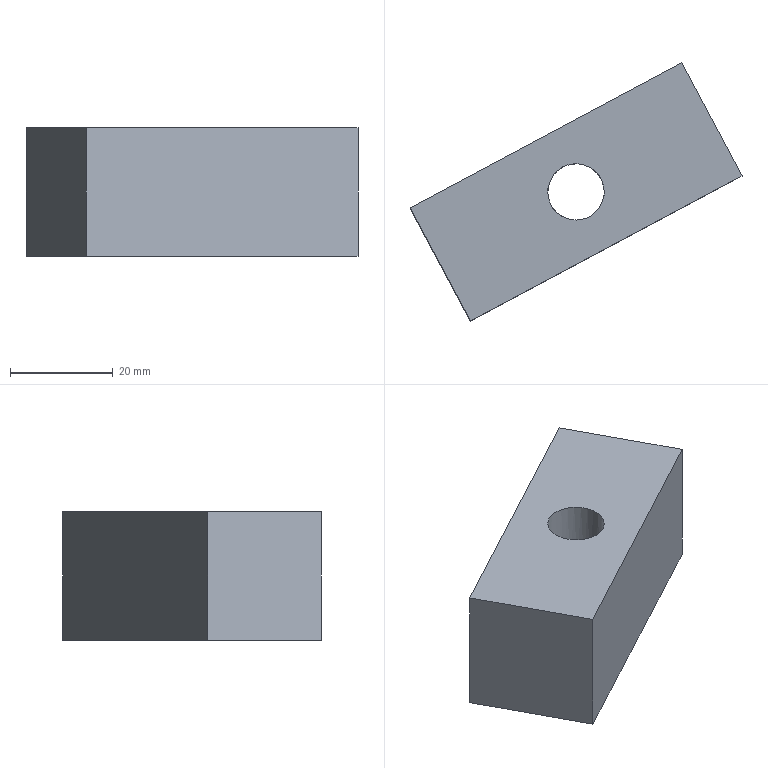Part | NX | features solid 2 | 1 solid | 9 faces | box 64.704 x 50.307 x 25 mm | volume 33211 mm3 | plane 7 | cylinder 2 | commonest cylinder face diameters 11 x1 18 x1
STEP:
#1=CARTESIAN_POINT('',(-802.083,-620.009,-2.));
#2=VERTEX_POINT('',#1);
#3=CARTESIAN_POINT('',(-749.151,-591.757,-2.));
#4=VERTEX_POINT('',#3);
#5=CARTESIAN_POINT('',(-802.083,-620.009,-2.));
#6=DIRECTION('',(0.8822,0.4709,0.));
#7=VECTOR('',#6,1000.);
#8=LINE('',#5,#7);
#9=EDGE_CURVE('',#2,#4,#8,.T.);
#10=ORIENTED_EDGE('',*,*,#9,.F.);
#11=CARTESIAN_POINT('',(-813.855,-597.954,-2.));
#12=VERTEX_POINT('',#11);
#13=CARTESIAN_POINT('',(-813.855,-597.954,-2.));
#14=DIRECTION('',(0.4709,-0.8822,0.));
#15=VECTOR('',#14,1000.);
#16=LINE('',#13,#15);
#17=EDGE_CURVE('',#12,#2,#16,.T.);
#18=ORIENTED_EDGE('',*,*,#17,.F.);
#19=CARTESIAN_POINT('',(-760.922,-569.702,-2.));
#20=VERTEX_POINT('',#19);
#21=CARTESIAN_POINT('',(-760.922,-569.702,-2.));
#22=DIRECTION('',(-0.8822,-0.4709,0.));
#23=VECTOR('',#22,1000.);
#24=LINE('',#21,#23);
#25=EDGE_CURVE('',#20,#12,#24,.T.);
#26=ORIENTED_EDGE('',*,*,#25,.F.);
#27=CARTESIAN_POINT('',(-749.151,-591.757,-2.));
#28=DIRECTION('',(-0.4709,0.8822,0.));
#29=VECTOR('',#28,1000.);
#30=LINE('',#27,#29);
#31=EDGE_CURVE('',#4,#20,#30,.T.);
#32=ORIENTED_EDGE('',*,*,#31,.F.);
#33=EDGE_LOOP('',(#10,#18,#26,#32));
#34=FACE_BOUND('',#33,.T.);
#35=CARTESIAN_POINT('',(-772.503,-594.855,-2.));
#36=VERTEX_POINT('',#35);
#37=CARTESIAN_POINT('',(-781.503,-594.855,-2.));
#38=DIRECTION('',(0.,0.,1.));
#39=DIRECTION('',(1.,0.,0.));
#40=AXIS2_PLACEMENT_3D('',#37,#38,#39);
#41=CIRCLE('',#40,9.);
#42=EDGE_CURVE('',#36,#36,#41,.F.);
#43=ORIENTED_EDGE('',*,*,#42,.F.);
#44=EDGE_LOOP('',(#43));
#45=FACE_BOUND('',#44,.T.);
#46=CARTESIAN_POINT('',(-749.151,-591.757,-2.));
#47=DIRECTION('',(0.,0.,-1.));
#48=DIRECTION('',(1.,0.,0.));
#49=AXIS2_PLACEMENT_3D('',#46,#47,#48);
#50=PLANE('',#49);
#51=ADVANCED_FACE('',(#34,#45),#50,.T.);
#52=CARTESIAN_POINT('',(-778.913,-599.707,23.));
#53=VERTEX_POINT('',#52);
#54=CARTESIAN_POINT('',(-781.503,-594.855,23.));
#55=DIRECTION('',(0.,0.,1.));
#56=DIRECTION('',(0.4709,-0.8822,0.));
#57=AXIS2_PLACEMENT_3D('',#54,#55,#56);
#58=CIRCLE('',#57,5.5);
#59=EDGE_CURVE('',#53,#53,#58,.T.);
#60=ORIENTED_EDGE('',*,*,#59,.T.);
#61=EDGE_LOOP('',(#60));
#62=FACE_BOUND('',#61,.T.);
#63=CARTESIAN_POINT('',(-776.003,-594.855,10.));
#64=VERTEX_POINT('',#63);
#65=CARTESIAN_POINT('',(-781.503,-594.855,10.));
#66=DIRECTION('',(0.,0.,1.));
#67=DIRECTION('',(1.,0.,0.));
#68=AXIS2_PLACEMENT_3D('',#65,#66,#67);
#69=CIRCLE('',#68,5.5);
#70=EDGE_CURVE('',#64,#64,#69,.T.);
#71=ORIENTED_EDGE('',*,*,#70,.F.);
#72=EDGE_LOOP('',(#71));
#73=FACE_BOUND('',#72,.T.);
#74=CARTESIAN_POINT('',(-781.503,-594.855,-2.));
#75=DIRECTION('',(0.,0.,1.));
#76=DIRECTION('',(-1.,0.,0.));
#77=AXIS2_PLACEMENT_3D('',#74,#75,#76);
#78=CYLINDRICAL_SURFACE('',#77,5.5);
#79=ADVANCED_FACE('',(#62,#73),#78,.F.);
#80=CARTESIAN_POINT('',(-802.083,-620.009,23.));
#81=VERTEX_POINT('',#80);
#82=CARTESIAN_POINT('',(-749.151,-591.757,23.));
#83=VERTEX_POINT('',#82);
#84=CARTESIAN_POINT('',(-802.083,-620.009,23.));
#85=DIRECTION('',(0.8822,0.4709,0.));
#86=VECTOR('',#85,1000.);
#87=LINE('',#84,#86);
#88=EDGE_CURVE('',#81,#83,#87,.T.);
#89=ORIENTED_EDGE('',*,*,#88,.T.);
#90=CARTESIAN_POINT('',(-760.922,-569.702,23.));
#91=VERTEX_POINT('',#90);
#92=CARTESIAN_POINT('',(-749.151,-591.757,23.));
#93=DIRECTION('',(-0.4709,0.8822,0.));
#94=VECTOR('',#93,1000.);
#95=LINE('',#92,#94);
#96=EDGE_CURVE('',#83,#91,#95,.T.);
#97=ORIENTED_EDGE('',*,*,#96,.T.);
#98=CARTESIAN_POINT('',(-813.855,-597.954,23.));
#99=VERTEX_POINT('',#98);
#100=CARTESIAN_POINT('',(-760.922,-569.702,23.));
#101=DIRECTION('',(-0.8822,-0.4709,0.));
#102=VECTOR('',#101,1000.);
#103=LINE('',#100,#102);
#104=EDGE_CURVE('',#91,#99,#103,.T.);
#105=ORIENTED_EDGE('',*,*,#104,.T.);
#106=CARTESIAN_POINT('',(-813.855,-597.954,23.));
#107=DIRECTION('',(0.4709,-0.8822,0.));
#108=VECTOR('',#107,1000.);
#109=LINE('',#106,#108);
#110=EDGE_CURVE('',#99,#81,#109,.T.);
#111=ORIENTED_EDGE('',*,*,#110,.T.);
#112=EDGE_LOOP('',(#89,#97,#105,#111));
#113=FACE_BOUND('',#112,.T.);
#114=ORIENTED_EDGE('',*,*,#59,.F.);
#115=EDGE_LOOP('',(#114));
#116=FACE_BOUND('',#115,.T.);
#117=CARTESIAN_POINT('',(-749.151,-591.757,23.));
#118=DIRECTION('',(0.,0.,-1.));
#119=DIRECTION('',(1.,0.,0.));
#120=AXIS2_PLACEMENT_3D('',#117,#118,#119);
#121=PLANE('',#120);
#122=ADVANCED_FACE('',(#113,#116),#121,.F.);
#123=ORIENTED_EDGE('',*,*,#88,.F.);
#124=CARTESIAN_POINT('',(-802.083,-620.009,-2.));
#125=DIRECTION('',(0.,0.,1.));
#126=VECTOR('',#125,1000.);
#127=LINE('',#124,#126);
#128=EDGE_CURVE('',#2,#81,#127,.T.);
#129=ORIENTED_EDGE('',*,*,#128,.F.);
#130=ORIENTED_EDGE('',*,*,#9,.T.);
#131=CARTESIAN_POINT('',(-749.151,-591.757,-2.));
#132=DIRECTION('',(0.,0.,1.));
#133=VECTOR('',#132,1000.);
#134=LINE('',#131,#133);
#135=EDGE_CURVE('',#4,#83,#134,.T.);
#136=ORIENTED_EDGE('',*,*,#135,.T.);
#137=EDGE_LOOP('',(#123,#129,#130,#136));
#138=FACE_BOUND('',#137,.T.);
#139=CARTESIAN_POINT('',(-802.083,-620.009,-2.));
#140=DIRECTION('',(-0.4709,0.8822,0.));
#141=DIRECTION('',(0.8822,0.4709,0.));
#142=AXIS2_PLACEMENT_3D('',#139,#140,#141);
#143=PLANE('',#142);
#144=ADVANCED_FACE('',(#138),#143,.F.);
#145=ORIENTED_EDGE('',*,*,#96,.F.);
#146=ORIENTED_EDGE('',*,*,#135,.F.);
#147=ORIENTED_EDGE('',*,*,#31,.T.);
#148=CARTESIAN_POINT('',(-760.922,-569.702,-2.));
#149=DIRECTION('',(0.,0.,1.));
#150=VECTOR('',#149,1000.);
#151=LINE('',#148,#150);
#152=EDGE_CURVE('',#20,#91,#151,.T.);
#153=ORIENTED_EDGE('',*,*,#152,.T.);
#154=EDGE_LOOP('',(#145,#146,#147,#153));
#155=FACE_BOUND('',#154,.T.);
#156=CARTESIAN_POINT('',(-749.151,-591.757,-2.));
#157=DIRECTION('',(-0.8822,-0.4709,0.));
#158=DIRECTION('',(-0.4709,0.8822,0.));
#159=AXIS2_PLACEMENT_3D('',#156,#157,#158);
#160=PLANE('',#159);
#161=ADVANCED_FACE('',(#155),#160,.F.);
#162=ORIENTED_EDGE('',*,*,#104,.F.);
#163=ORIENTED_EDGE('',*,*,#152,.F.);
#164=ORIENTED_EDGE('',*,*,#25,.T.);
#165=CARTESIAN_POINT('',(-813.855,-597.954,-2.));
#166=DIRECTION('',(0.,0.,1.));
#167=VECTOR('',#166,1000.);
#168=LINE('',#165,#167);
#169=EDGE_CURVE('',#12,#99,#168,.T.);
#170=ORIENTED_EDGE('',*,*,#169,.T.);
#171=EDGE_LOOP('',(#162,#163,#164,#170));
#172=FACE_BOUND('',#171,.T.);
#173=CARTESIAN_POINT('',(-760.922,-569.702,-2.));
#174=DIRECTION('',(0.4709,-0.8822,0.));
#175=DIRECTION('',(-0.8822,-0.4709,0.));
#176=AXIS2_PLACEMENT_3D('',#173,#174,#175);
#177=PLANE('',#176);
#178=ADVANCED_FACE('',(#172),#177,.F.);
#179=ORIENTED_EDGE('',*,*,#110,.F.);
#180=ORIENTED_EDGE('',*,*,#169,.F.);
#181=ORIENTED_EDGE('',*,*,#17,.T.);
#182=ORIENTED_EDGE('',*,*,#128,.T.);
#183=EDGE_LOOP('',(#179,#180,#181,#182));
#184=FACE_BOUND('',#183,.T.);
#185=CARTESIAN_POINT('',(-813.855,-597.954,-2.));
#186=DIRECTION('',(0.8822,0.4709,0.));
#187=DIRECTION('',(0.4709,-0.8822,0.));
#188=AXIS2_PLACEMENT_3D('',#185,#186,#187);
#189=PLANE('',#188);
#190=ADVANCED_FACE('',(#184),#189,.F.);
#191=ORIENTED_EDGE('',*,*,#42,.T.);
#192=EDGE_LOOP('',(#191));
#193=FACE_BOUND('',#192,.T.);
#194=CARTESIAN_POINT('',(-777.265,-602.795,10.));
#195=VERTEX_POINT('',#194);
#196=CARTESIAN_POINT('',(-781.503,-594.855,10.));
#197=DIRECTION('',(0.,0.,1.));
#198=DIRECTION('',(0.4709,-0.8822,0.));
#199=AXIS2_PLACEMENT_3D('',#196,#197,#198);
#200=CIRCLE('',#199,9.);
#201=EDGE_CURVE('',#195,#195,#200,.T.);
#202=ORIENTED_EDGE('',*,*,#201,.T.);
#203=EDGE_LOOP('',(#202));
#204=FACE_BOUND('',#203,.T.);
#205=CARTESIAN_POINT('',(-781.503,-594.855,-15.));
#206=DIRECTION('',(0.,0.,1.));
#207=DIRECTION('',(-1.,0.,0.));
#208=AXIS2_PLACEMENT_3D('',#205,#206,#207);
#209=CYLINDRICAL_SURFACE('',#208,9.);
#210=ADVANCED_FACE('',(#193,#204),#209,.F.);
#211=ORIENTED_EDGE('',*,*,#70,.T.);
#212=EDGE_LOOP('',(#211));
#213=FACE_BOUND('',#212,.T.);
#214=ORIENTED_EDGE('',*,*,#201,.F.);
#215=EDGE_LOOP('',(#214));
#216=FACE_BOUND('',#215,.T.);
#217=CARTESIAN_POINT('',(-781.503,-594.855,10.));
#218=DIRECTION('',(0.,0.,-1.));
#219=DIRECTION('',(1.,0.,0.));
#220=AXIS2_PLACEMENT_3D('',#217,#218,#219);
#221=PLANE('',#220);
#222=ADVANCED_FACE('',(#213,#216),#221,.T.);
#223=CLOSED_SHELL('',(#51,#79,#122,#144,#161,#178,#190,#210,#222));
#224=MANIFOLD_SOLID_BREP('',#223);
#225=(LENGTH_UNIT()NAMED_UNIT(*)SI_UNIT(.MILLI.,.METRE.));
#226=UNCERTAINTY_MEASURE_WITH_UNIT(LENGTH_MEASURE(0.00001),#225,'','');
#227=(NAMED_UNIT(*)PLANE_ANGLE_UNIT()SI_UNIT($,.RADIAN.));
#228=(NAMED_UNIT(*)SI_UNIT($,.STERADIAN.)SOLID_ANGLE_UNIT());
#229=(GEOMETRIC_REPRESENTATION_CONTEXT(3)GLOBAL_UNCERTAINTY_ASSIGNED_CONTEXT((#226))GLOBAL_UNIT_ASSIGNED_CONTEXT((#225,#227,#228))REPRESENTATION_CONTEXT('',''));
#230=ADVANCED_BREP_SHAPE_REPRESENTATION('',(#224),#229);